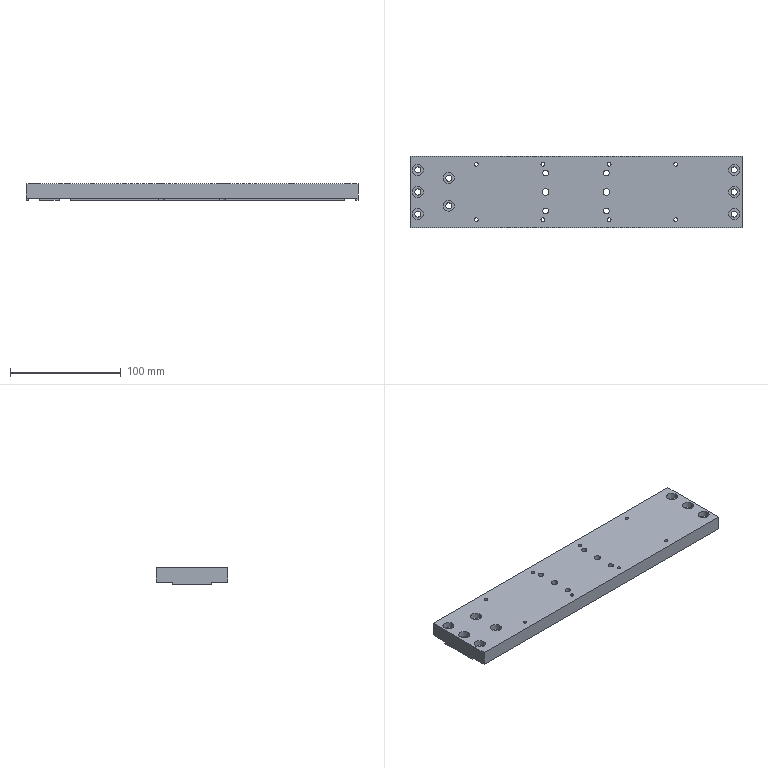Part | STEP file | A07 | 1 solid | 96 faces | box 300 x 65 x 15 mm | volume 264705 mm3 | cylinder 60 | plane 36 | commonest cylinder face diameters 3.3 x16 5.5 x16 10 x16 5 x8 6 x4